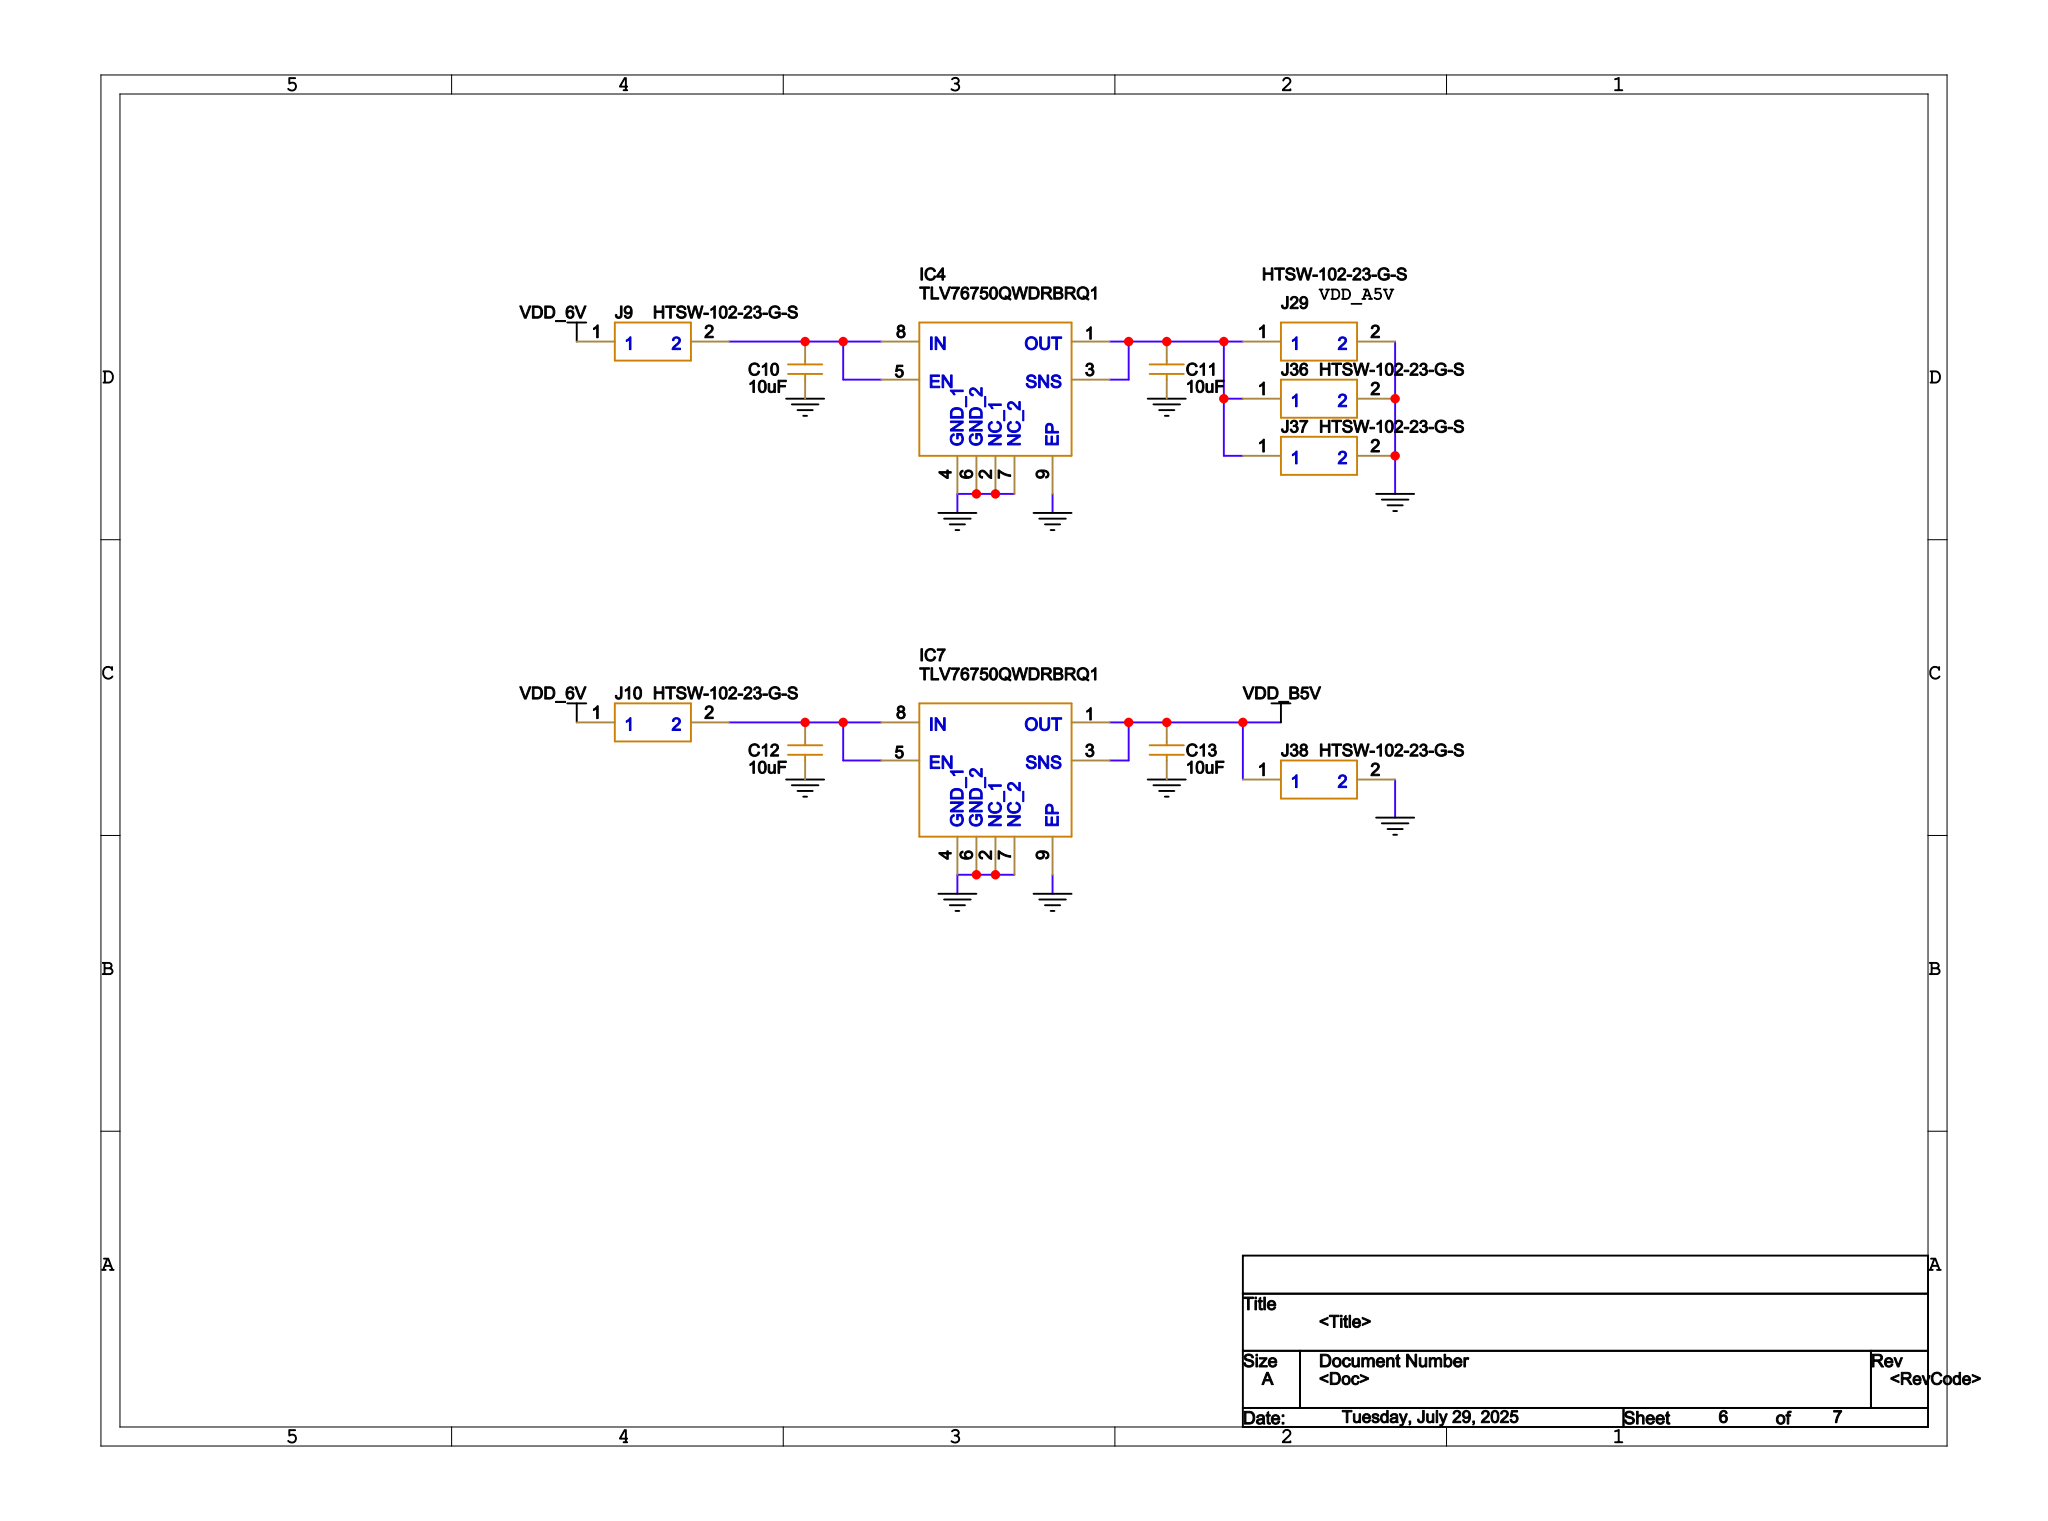Circuit board | Cadence Allegro | 93 parts | 49 nets | one sheet of the schematic
Parts on this sheet (reference | value | footprint):
C10 | 10uF | C1210
C11 | 10uF | C1210
C12 | 10uF | C1210
C13 | 10uF | C1210
IC4 | TLV76750QWDRBRQ1 | SON65P300X300X100-9N-D
IC7 | TLV76750QWDRBRQ1 | SON65P300X300X100-9N-D
J9 | HTSW-102-23-G-S | HDRV2W64P0X254_1X2_508X248X838P
J10 | HTSW-102-23-G-S | HDRV2W64P0X254_1X2_508X248X838P
J29 | HTSW-102-23-G-S | HDRV2W64P0X254_1X2_508X248X838P
J36 | HTSW-102-23-G-S | HDRV2W64P0X254_1X2_508X248X838P
J37 | HTSW-102-23-G-S | HDRV2W64P0X254_1X2_508X248X838P
J38 | HTSW-102-23-G-S | HDRV2W64P0X254_1X2_508X248X838P
Nets of these parts (net: part-pin ...):
VDD_6V: J9-1 J10-1
GND: C10-2 C11-2 C12-2 C13-2 IC4-2 IC4-4 IC4-6 IC4-7 IC4-9 IC7-2 IC7-4 IC7-6 IC7-7 IC7-9 J29-2 J36-2 J37-2 J38-2
N05480: C10-1 IC4-5 IC4-8 J9-2
N05704: C11-1 IC4-1 IC4-3 J29-1 J36-1 J37-1
N06176: C12-1 IC7-5 IC7-8 J10-2
VDD_B5V: C13-1 IC7-1 IC7-3 J38-1